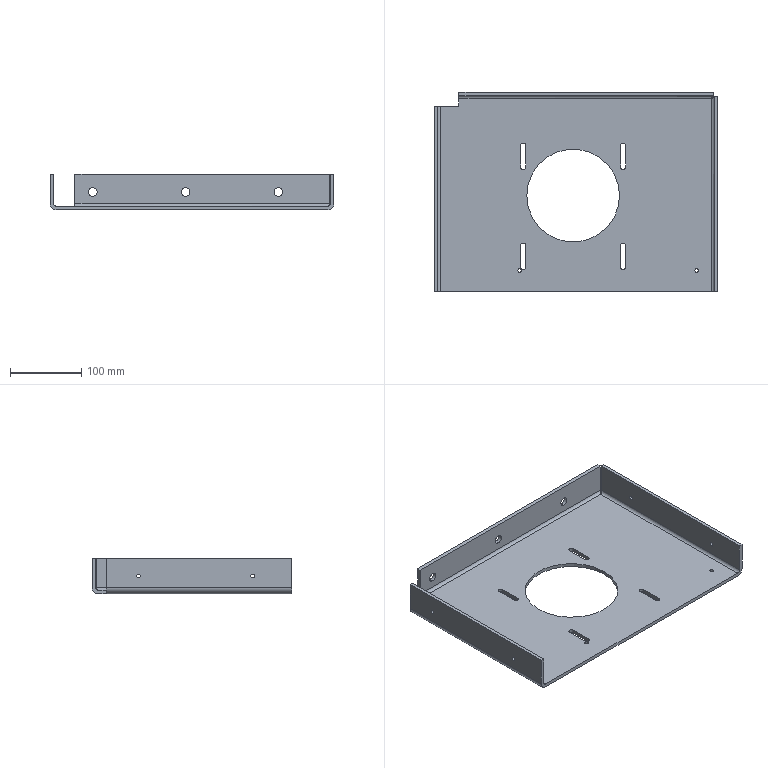Part | STEP file | PN_0029_side plate_default_machined_ | 1 solid | 60 faces | box 398 x 280 x 50 mm | volume 667972 mm3 | cylinder 34 | plane 24 | spline 2 | commonest cylinder face diameters 5 x12 7 x8 12 x6 8 x3 18 x3 130 x2